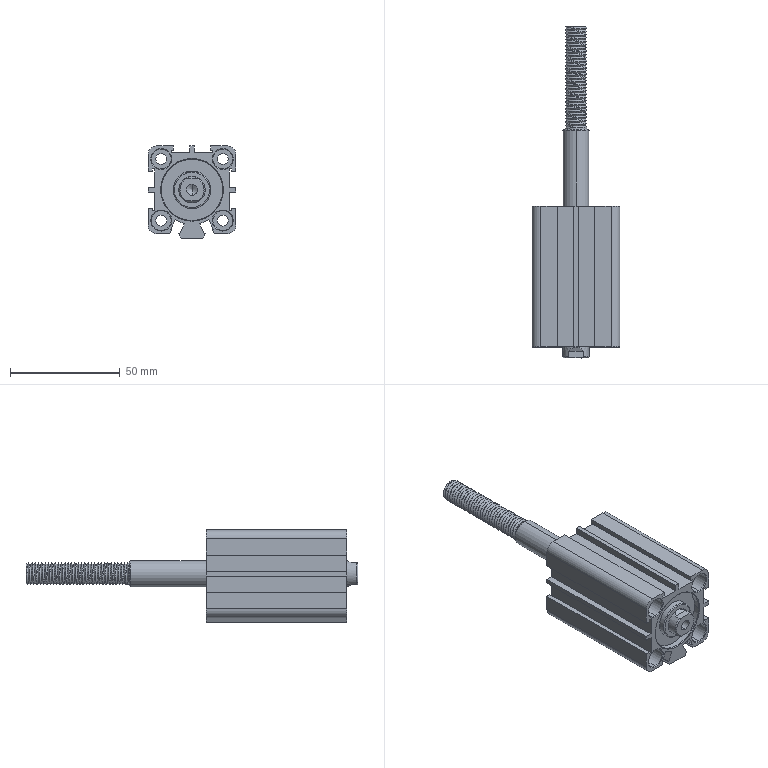Part | STEP file | Air cylinder ACQJ-25X35-20_4_1-5 | 1 solid | 182 faces | box 40 x 151.001 x 42 mm | volume 88087 mm3 | plane 78 | cylinder 47 | cone 34 | spline 23 | commonest cylinder face diameters 9 x16 5 x10 4.2 x4 8 x4 12 x4 17 x4